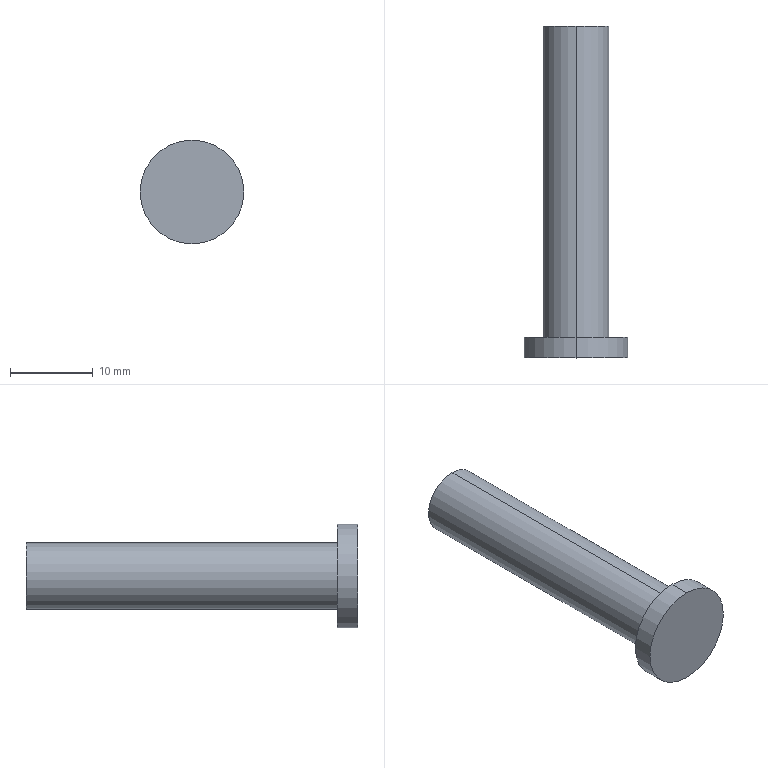Part | SolidWorks | features Revolution 1 | 1 solid | 7 faces | box 12.5 x 40 x 12.5 mm | volume 2192 mm3 | cylinder 4 | plane 3 | commonest cylinder face diameters 8 x2 12.5 x2
STEP:
#1=CARTESIAN_POINT('',(0.,-37.5,-6.25));
#2=VERTEX_POINT('',#1);
#3=CARTESIAN_POINT('',(0.,-37.5,6.25));
#4=VERTEX_POINT('',#3);
#5=CARTESIAN_POINT('',(0.,-37.5,0.));
#6=DIRECTION('',(0.,-1.,0.));
#7=DIRECTION('',(0.,0.,-1.));
#8=AXIS2_PLACEMENT_3D('',#5,#6,#7);
#9=CIRCLE('',#8,6.25);
#10=EDGE_CURVE('',#2,#4,#9,.T.);
#11=ORIENTED_EDGE('',*,*,#10,.T.);
#12=CARTESIAN_POINT('',(0.,-40.,6.25));
#13=VERTEX_POINT('',#12);
#14=CARTESIAN_POINT('',(0.,-40.,6.25));
#15=DIRECTION('',(0.,-1.,0.));
#16=VECTOR('',#15,1000.);
#17=LINE('',#14,#16);
#18=EDGE_CURVE('',#4,#13,#17,.T.);
#19=ORIENTED_EDGE('',*,*,#18,.T.);
#20=CARTESIAN_POINT('',(0.,-40.,-6.25));
#21=VERTEX_POINT('',#20);
#22=CARTESIAN_POINT('',(0.,-40.,0.));
#23=DIRECTION('',(0.,-1.,0.));
#24=DIRECTION('',(0.,0.,-1.));
#25=AXIS2_PLACEMENT_3D('',#22,#23,#24);
#26=CIRCLE('',#25,6.25);
#27=EDGE_CURVE('',#21,#13,#26,.T.);
#28=ORIENTED_EDGE('',*,*,#27,.F.);
#29=CARTESIAN_POINT('',(0.,-40.,-6.25));
#30=DIRECTION('',(0.,-1.,0.));
#31=VECTOR('',#30,1000.);
#32=LINE('',#29,#31);
#33=EDGE_CURVE('',#2,#21,#32,.T.);
#34=ORIENTED_EDGE('',*,*,#33,.F.);
#35=EDGE_LOOP('',(#11,#19,#28,#34));
#36=FACE_OUTER_BOUND('',#35,.T.);
#37=CARTESIAN_POINT('',(0.,-40.,0.));
#38=DIRECTION('',(0.,-1.,0.));
#39=DIRECTION('',(0.,0.,-1.));
#40=AXIS2_PLACEMENT_3D('',#37,#38,#39);
#41=CYLINDRICAL_SURFACE('',#40,6.25);
#42=ADVANCED_FACE('',(#36),#41,.T.);
#43=CARTESIAN_POINT('',(0.,0.,-4.));
#44=VERTEX_POINT('',#43);
#45=CARTESIAN_POINT('',(0.,0.,4.));
#46=VERTEX_POINT('',#45);
#47=CARTESIAN_POINT('',(0.,0.,0.));
#48=DIRECTION('',(0.,-1.,0.));
#49=DIRECTION('',(0.,0.,-1.));
#50=AXIS2_PLACEMENT_3D('',#47,#48,#49);
#51=CIRCLE('',#50,4.);
#52=EDGE_CURVE('',#44,#46,#51,.T.);
#53=ORIENTED_EDGE('',*,*,#52,.T.);
#54=CARTESIAN_POINT('',(0.,-37.5,4.));
#55=VERTEX_POINT('',#54);
#56=CARTESIAN_POINT('',(0.,-40.,4.));
#57=DIRECTION('',(0.,-1.,0.));
#58=VECTOR('',#57,1000.);
#59=LINE('',#56,#58);
#60=EDGE_CURVE('',#46,#55,#59,.T.);
#61=ORIENTED_EDGE('',*,*,#60,.T.);
#62=CARTESIAN_POINT('',(0.,-37.5,-4.));
#63=VERTEX_POINT('',#62);
#64=CARTESIAN_POINT('',(0.,-37.5,0.));
#65=DIRECTION('',(0.,-1.,0.));
#66=DIRECTION('',(0.,0.,-1.));
#67=AXIS2_PLACEMENT_3D('',#64,#65,#66);
#68=CIRCLE('',#67,4.);
#69=EDGE_CURVE('',#63,#55,#68,.T.);
#70=ORIENTED_EDGE('',*,*,#69,.F.);
#71=CARTESIAN_POINT('',(0.,-40.,-4.));
#72=DIRECTION('',(0.,-1.,0.));
#73=VECTOR('',#72,1000.);
#74=LINE('',#71,#73);
#75=EDGE_CURVE('',#44,#63,#74,.T.);
#76=ORIENTED_EDGE('',*,*,#75,.F.);
#77=EDGE_LOOP('',(#53,#61,#70,#76));
#78=FACE_OUTER_BOUND('',#77,.T.);
#79=CARTESIAN_POINT('',(0.,-40.,0.));
#80=DIRECTION('',(0.,-1.,0.));
#81=DIRECTION('',(0.,0.,-1.));
#82=AXIS2_PLACEMENT_3D('',#79,#80,#81);
#83=CYLINDRICAL_SURFACE('',#82,4.);
#84=ADVANCED_FACE('',(#78),#83,.T.);
#85=ORIENTED_EDGE('',*,*,#52,.F.);
#86=CARTESIAN_POINT('',(0.,0.,0.));
#87=DIRECTION('',(0.,-1.,0.));
#88=DIRECTION('',(0.,0.,-1.));
#89=AXIS2_PLACEMENT_3D('',#86,#87,#88);
#90=CIRCLE('',#89,4.);
#91=EDGE_CURVE('',#46,#44,#90,.T.);
#92=ORIENTED_EDGE('',*,*,#91,.F.);
#93=EDGE_LOOP('',(#85,#92));
#94=FACE_OUTER_BOUND('',#93,.T.);
#95=CARTESIAN_POINT('',(0.,0.,0.));
#96=DIRECTION('',(0.,1.,0.));
#97=DIRECTION('',(0.,0.,1.));
#98=AXIS2_PLACEMENT_3D('',#95,#96,#97);
#99=PLANE('',#98);
#100=ADVANCED_FACE('',(#94),#99,.T.);
#101=ORIENTED_EDGE('',*,*,#60,.F.);
#102=ORIENTED_EDGE('',*,*,#91,.T.);
#103=ORIENTED_EDGE('',*,*,#75,.T.);
#104=CARTESIAN_POINT('',(0.,-37.5,0.));
#105=DIRECTION('',(0.,-1.,0.));
#106=DIRECTION('',(0.,0.,-1.));
#107=AXIS2_PLACEMENT_3D('',#104,#105,#106);
#108=CIRCLE('',#107,4.);
#109=EDGE_CURVE('',#55,#63,#108,.T.);
#110=ORIENTED_EDGE('',*,*,#109,.F.);
#111=EDGE_LOOP('',(#101,#102,#103,#110));
#112=FACE_OUTER_BOUND('',#111,.T.);
#113=CARTESIAN_POINT('',(0.,-40.,0.));
#114=DIRECTION('',(0.,-1.,0.));
#115=DIRECTION('',(0.,0.,-1.));
#116=AXIS2_PLACEMENT_3D('',#113,#114,#115);
#117=CYLINDRICAL_SURFACE('',#116,4.);
#118=ADVANCED_FACE('',(#112),#117,.T.);
#119=ORIENTED_EDGE('',*,*,#69,.T.);
#120=ORIENTED_EDGE('',*,*,#109,.T.);
#121=EDGE_LOOP('',(#119,#120));
#122=FACE_BOUND('',#121,.T.);
#123=ORIENTED_EDGE('',*,*,#10,.F.);
#124=CARTESIAN_POINT('',(0.,-37.5,0.));
#125=DIRECTION('',(0.,-1.,0.));
#126=DIRECTION('',(0.,0.,-1.));
#127=AXIS2_PLACEMENT_3D('',#124,#125,#126);
#128=CIRCLE('',#127,6.25);
#129=EDGE_CURVE('',#4,#2,#128,.T.);
#130=ORIENTED_EDGE('',*,*,#129,.F.);
#131=EDGE_LOOP('',(#123,#130));
#132=FACE_OUTER_BOUND('',#131,.T.);
#133=CARTESIAN_POINT('',(4.,-37.5,0.));
#134=DIRECTION('',(0.,1.,0.));
#135=DIRECTION('',(0.,0.,1.));
#136=AXIS2_PLACEMENT_3D('',#133,#134,#135);
#137=PLANE('',#136);
#138=ADVANCED_FACE('',(#122,#132),#137,.T.);
#139=ORIENTED_EDGE('',*,*,#18,.F.);
#140=ORIENTED_EDGE('',*,*,#129,.T.);
#141=ORIENTED_EDGE('',*,*,#33,.T.);
#142=CARTESIAN_POINT('',(0.,-40.,0.));
#143=DIRECTION('',(0.,-1.,0.));
#144=DIRECTION('',(0.,0.,-1.));
#145=AXIS2_PLACEMENT_3D('',#142,#143,#144);
#146=CIRCLE('',#145,6.25);
#147=EDGE_CURVE('',#13,#21,#146,.T.);
#148=ORIENTED_EDGE('',*,*,#147,.F.);
#149=EDGE_LOOP('',(#139,#140,#141,#148));
#150=FACE_OUTER_BOUND('',#149,.T.);
#151=CARTESIAN_POINT('',(0.,-40.,0.));
#152=DIRECTION('',(0.,-1.,0.));
#153=DIRECTION('',(0.,0.,-1.));
#154=AXIS2_PLACEMENT_3D('',#151,#152,#153);
#155=CYLINDRICAL_SURFACE('',#154,6.25);
#156=ADVANCED_FACE('',(#150),#155,.T.);
#157=ORIENTED_EDGE('',*,*,#27,.T.);
#158=ORIENTED_EDGE('',*,*,#147,.T.);
#159=EDGE_LOOP('',(#157,#158));
#160=FACE_OUTER_BOUND('',#159,.T.);
#161=CARTESIAN_POINT('',(6.25,-40.,0.));
#162=DIRECTION('',(0.,-1.,0.));
#163=DIRECTION('',(0.,0.,-1.));
#164=AXIS2_PLACEMENT_3D('',#161,#162,#163);
#165=PLANE('',#164);
#166=ADVANCED_FACE('',(#160),#165,.T.);
#167=CLOSED_SHELL('',(#42,#84,#100,#118,#138,#156,#166));
#168=MANIFOLD_SOLID_BREP('',#167);
#169=CARTESIAN_POINT('',(0.,0.,0.));
#170=DIRECTION('',(0.,0.,1.));
#171=DIRECTION('',(1.,0.,0.));
#172=AXIS2_PLACEMENT_3D('',#169,#170,#171);
#173=(LENGTH_UNIT()NAMED_UNIT(*)SI_UNIT(.MILLI.,.METRE.));
#174=UNCERTAINTY_MEASURE_WITH_UNIT(LENGTH_MEASURE(0.00001),#173,'','');
#175=(NAMED_UNIT(*)PLANE_ANGLE_UNIT()SI_UNIT($,.RADIAN.));
#176=(NAMED_UNIT(*)SI_UNIT($,.STERADIAN.)SOLID_ANGLE_UNIT());
#177=(GEOMETRIC_REPRESENTATION_CONTEXT(3)GLOBAL_UNCERTAINTY_ASSIGNED_CONTEXT((#174))GLOBAL_UNIT_ASSIGNED_CONTEXT((#173,#175,#176))REPRESENTATION_CONTEXT('',''));
#178=ADVANCED_BREP_SHAPE_REPRESENTATION('',(#168,#172),#177);